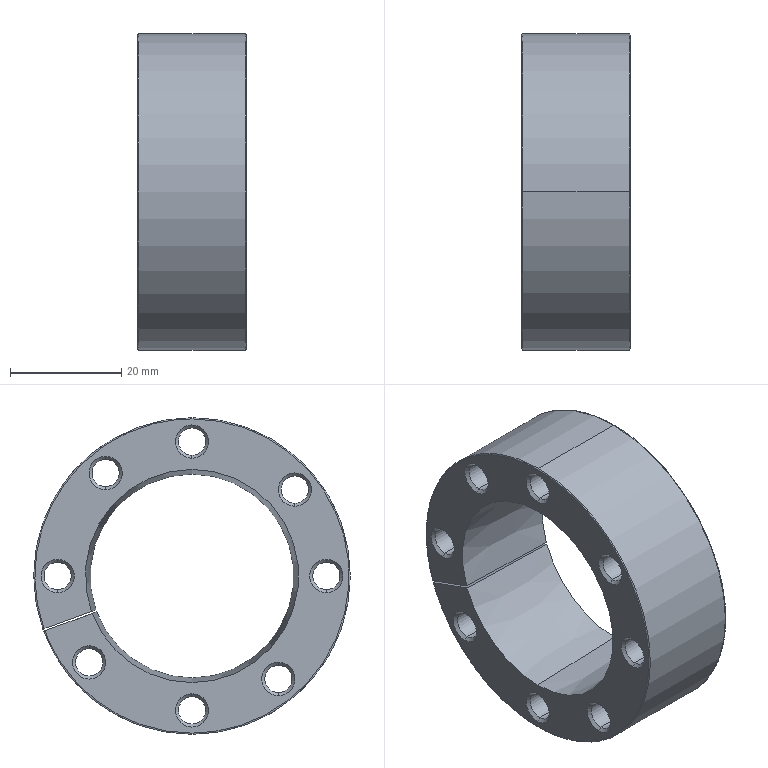Part | STEP file | expansion sleeve A^PN_0025_expansion sleeve | 1 solid | 64 faces | box 19.5 x 57 x 57 mm | volume 25082 mm3 | cone 35 | cylinder 19 | spline 6 | plane 4 | commonest cylinder face diameters 4.917 x16 57 x3